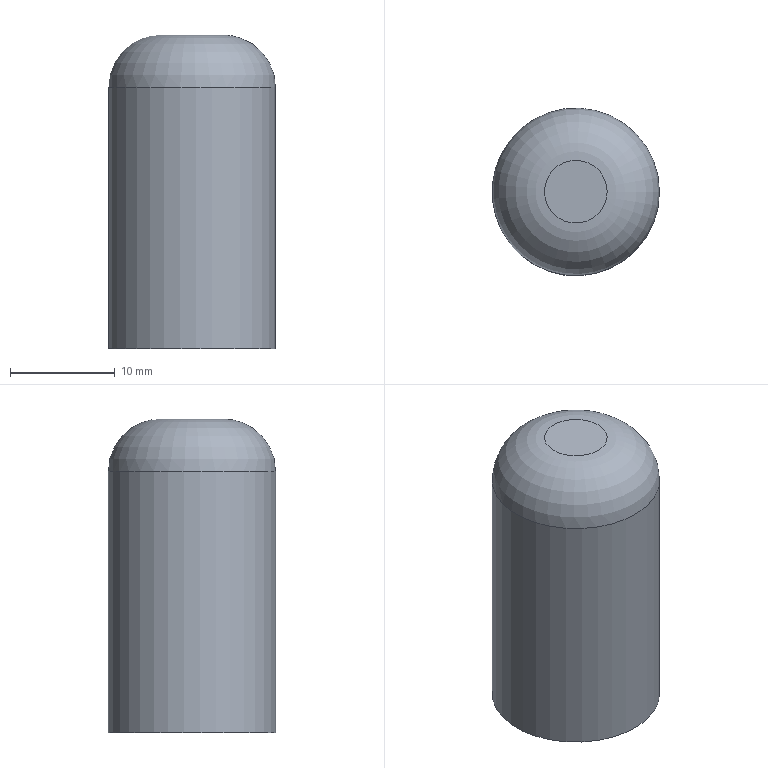Part | NX | features DATUM_CSYS 2, BLEND 1, EXTRUDE 1, SHELL 1, SKETCH 1 | 1 solid | 7 faces | box 16 x 16 x 30 mm | volume 1467 mm3 | plane 3 | cylinder 2 | torus 2 | commonest cylinder face diameters 14 x1 16 x1
STEP:
#1=CARTESIAN_POINT('',(8.,0.,25.));
#2=VERTEX_POINT('',#1);
#3=CARTESIAN_POINT('',(0.,0.,25.));
#4=DIRECTION('',(0.,0.,1.));
#5=DIRECTION('',(1.,0.,0.));
#6=AXIS2_PLACEMENT_3D('',#3,#4,#5);
#7=CIRCLE('',#6,8.);
#8=EDGE_CURVE('',#2,#2,#7,.F.);
#9=ORIENTED_EDGE('',*,*,#8,.T.);
#10=EDGE_LOOP('',(#9));
#11=FACE_BOUND('',#10,.T.);
#12=CARTESIAN_POINT('',(8.,0.,0.));
#13=VERTEX_POINT('',#12);
#14=CARTESIAN_POINT('',(0.,0.,0.));
#15=DIRECTION('',(0.,0.,1.));
#16=DIRECTION('',(1.,0.,0.));
#17=AXIS2_PLACEMENT_3D('',#14,#15,#16);
#18=CIRCLE('',#17,8.);
#19=EDGE_CURVE('',#13,#13,#18,.T.);
#20=ORIENTED_EDGE('',*,*,#19,.T.);
#21=EDGE_LOOP('',(#20));
#22=FACE_BOUND('',#21,.T.);
#23=CARTESIAN_POINT('',(0.,0.,30.));
#24=DIRECTION('',(0.,0.,-1.));
#25=DIRECTION('',(-1.,0.,0.));
#26=AXIS2_PLACEMENT_3D('',#23,#24,#25);
#27=CYLINDRICAL_SURFACE('',#26,8.);
#28=ADVANCED_FACE('',(#11,#22),#27,.T.);
#29=CARTESIAN_POINT('',(3.,0.,30.));
#30=VERTEX_POINT('',#29);
#31=CARTESIAN_POINT('',(0.,0.,30.));
#32=DIRECTION('',(0.,0.,1.));
#33=DIRECTION('',(1.,0.,0.));
#34=AXIS2_PLACEMENT_3D('',#31,#32,#33);
#35=CIRCLE('',#34,3.);
#36=EDGE_CURVE('',#30,#30,#35,.T.);
#37=ORIENTED_EDGE('',*,*,#36,.T.);
#38=EDGE_LOOP('',(#37));
#39=FACE_BOUND('',#38,.T.);
#40=CARTESIAN_POINT('',(0.,0.,30.));
#41=DIRECTION('',(0.,0.,1.));
#42=DIRECTION('',(1.,0.,0.));
#43=AXIS2_PLACEMENT_3D('',#40,#41,#42);
#44=PLANE('',#43);
#45=ADVANCED_FACE('',(#39),#44,.T.);
#46=CARTESIAN_POINT('',(7.,0.,0.));
#47=VERTEX_POINT('',#46);
#48=CARTESIAN_POINT('',(0.,0.,0.));
#49=DIRECTION('',(0.,0.,1.));
#50=DIRECTION('',(1.,0.,0.));
#51=AXIS2_PLACEMENT_3D('',#48,#49,#50);
#52=CIRCLE('',#51,7.);
#53=EDGE_CURVE('',#47,#47,#52,.T.);
#54=ORIENTED_EDGE('',*,*,#53,.T.);
#55=EDGE_LOOP('',(#54));
#56=FACE_BOUND('',#55,.T.);
#57=ORIENTED_EDGE('',*,*,#19,.F.);
#58=EDGE_LOOP('',(#57));
#59=FACE_BOUND('',#58,.T.);
#60=CARTESIAN_POINT('',(0.,0.,0.));
#61=DIRECTION('',(0.,0.,1.));
#62=DIRECTION('',(1.,0.,0.));
#63=AXIS2_PLACEMENT_3D('',#60,#61,#62);
#64=PLANE('',#63);
#65=ADVANCED_FACE('',(#56,#59),#64,.F.);
#66=ORIENTED_EDGE('',*,*,#8,.F.);
#67=EDGE_LOOP('',(#66));
#68=FACE_BOUND('',#67,.T.);
#69=ORIENTED_EDGE('',*,*,#36,.F.);
#70=EDGE_LOOP('',(#69));
#71=FACE_BOUND('',#70,.T.);
#72=CARTESIAN_POINT('',(0.,0.,25.));
#73=DIRECTION('',(0.,0.,1.));
#74=DIRECTION('',(1.,0.,0.));
#75=AXIS2_PLACEMENT_3D('',#72,#73,#74);
#76=DEGENERATE_TOROIDAL_SURFACE('',#75,3.,5.,.T.);
#77=ADVANCED_FACE('',(#68,#71),#76,.T.);
#78=CARTESIAN_POINT('',(-7.,0.,25.));
#79=VERTEX_POINT('',#78);
#80=CARTESIAN_POINT('',(0.,0.,25.));
#81=DIRECTION('',(0.,0.,-1.));
#82=DIRECTION('',(-1.,0.,0.));
#83=AXIS2_PLACEMENT_3D('',#80,#81,#82);
#84=CIRCLE('',#83,7.);
#85=EDGE_CURVE('',#79,#79,#84,.T.);
#86=ORIENTED_EDGE('',*,*,#85,.F.);
#87=EDGE_LOOP('',(#86));
#88=FACE_BOUND('',#87,.T.);
#89=ORIENTED_EDGE('',*,*,#53,.F.);
#90=EDGE_LOOP('',(#89));
#91=FACE_BOUND('',#90,.T.);
#92=CARTESIAN_POINT('',(0.,0.,30.));
#93=DIRECTION('',(0.,0.,-1.));
#94=DIRECTION('',(-1.,0.,0.));
#95=AXIS2_PLACEMENT_3D('',#92,#93,#94);
#96=CYLINDRICAL_SURFACE('',#95,7.);
#97=ADVANCED_FACE('',(#88,#91),#96,.F.);
#98=CARTESIAN_POINT('',(3.,0.,29.));
#99=VERTEX_POINT('',#98);
#100=CARTESIAN_POINT('',(0.,0.,29.));
#101=DIRECTION('',(0.,0.,1.));
#102=DIRECTION('',(1.,0.,0.));
#103=AXIS2_PLACEMENT_3D('',#100,#101,#102);
#104=CIRCLE('',#103,3.);
#105=EDGE_CURVE('',#99,#99,#104,.T.);
#106=ORIENTED_EDGE('',*,*,#105,.F.);
#107=EDGE_LOOP('',(#106));
#108=FACE_BOUND('',#107,.T.);
#109=CARTESIAN_POINT('',(0.,0.,29.));
#110=DIRECTION('',(0.,0.,1.));
#111=DIRECTION('',(1.,0.,0.));
#112=AXIS2_PLACEMENT_3D('',#109,#110,#111);
#113=PLANE('',#112);
#114=ADVANCED_FACE('',(#108),#113,.F.);
#115=ORIENTED_EDGE('',*,*,#85,.T.);
#116=EDGE_LOOP('',(#115));
#117=FACE_BOUND('',#116,.T.);
#118=ORIENTED_EDGE('',*,*,#105,.T.);
#119=EDGE_LOOP('',(#118));
#120=FACE_BOUND('',#119,.T.);
#121=CARTESIAN_POINT('',(0.,0.,25.));
#122=DIRECTION('',(0.,0.,1.));
#123=DIRECTION('',(1.,0.,0.));
#124=AXIS2_PLACEMENT_3D('',#121,#122,#123);
#125=DEGENERATE_TOROIDAL_SURFACE('',#124,3.,4.,.T.);
#126=ADVANCED_FACE('',(#117,#120),#125,.F.);
#127=CLOSED_SHELL('',(#28,#45,#65,#77,#97,#114,#126));
#128=MANIFOLD_SOLID_BREP('',#127);
#129=(LENGTH_UNIT()NAMED_UNIT(*)SI_UNIT(.MILLI.,.METRE.));
#130=UNCERTAINTY_MEASURE_WITH_UNIT(LENGTH_MEASURE(0.00001),#129,'','');
#131=(NAMED_UNIT(*)PLANE_ANGLE_UNIT()SI_UNIT($,.RADIAN.));
#132=(NAMED_UNIT(*)SI_UNIT($,.STERADIAN.)SOLID_ANGLE_UNIT());
#133=(GEOMETRIC_REPRESENTATION_CONTEXT(3)GLOBAL_UNCERTAINTY_ASSIGNED_CONTEXT((#130))GLOBAL_UNIT_ASSIGNED_CONTEXT((#129,#131,#132))REPRESENTATION_CONTEXT('',''));
#134=ADVANCED_BREP_SHAPE_REPRESENTATION('',(#128),#133);